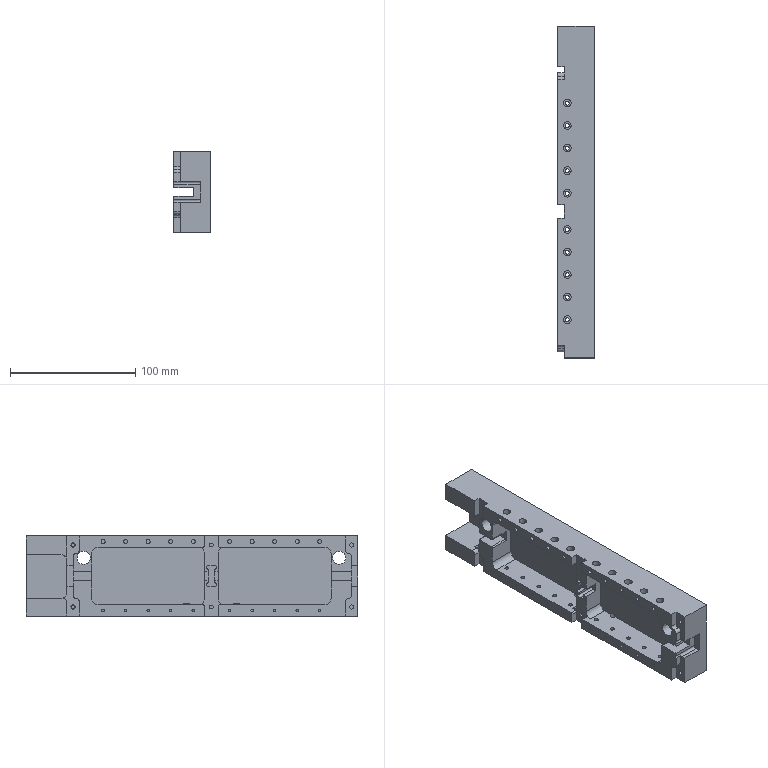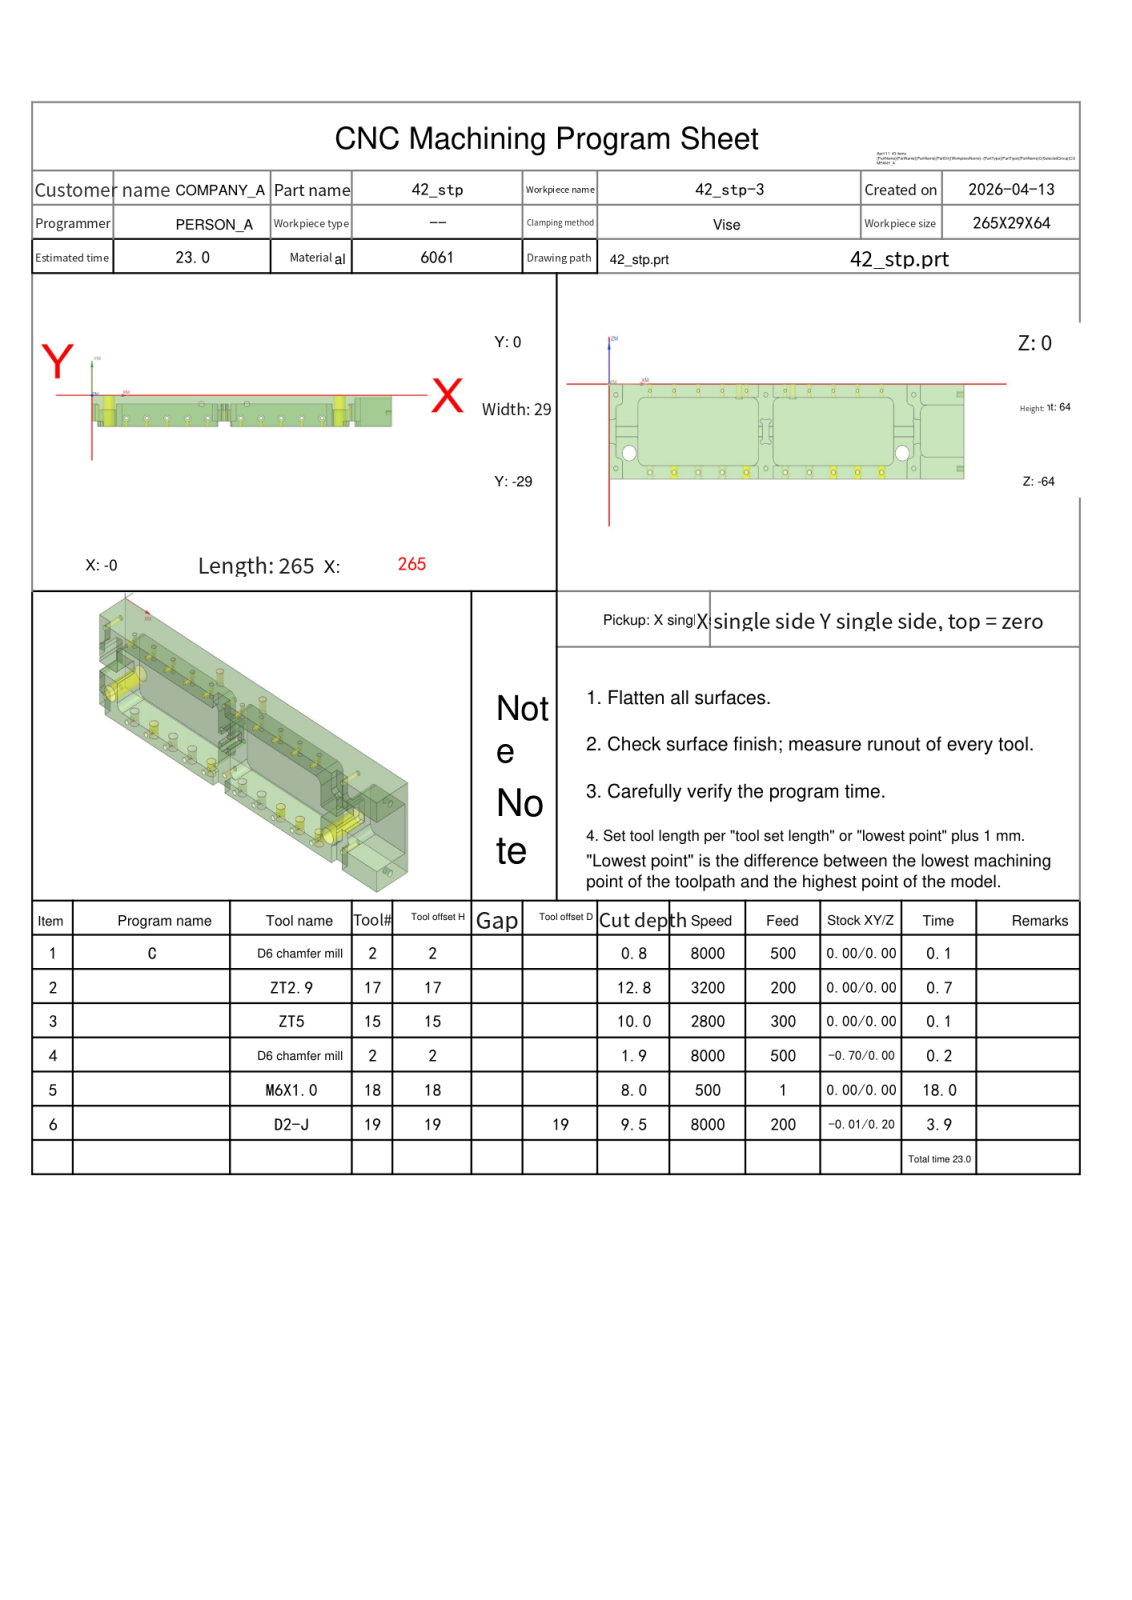NC program | NX | posted by the shop | part box 29 x 265 x 64 mm
Whole program:
%
O0001
(Machine time: 40.11 MIN)
(===Total Tool:5===)
(T2=D6 chamfer mill   D=6.   R=0.   D-  H02 Z=-1.85 )
(T17=ZT2.9  D=2.9  DR_a=120 D-  H17 Z=-12.84)
(T15=ZT5    D=5.   DR_a=118 D-  H15 Z=-10.  )
(T18=M6X1.0 D=5.   DR_a=180 D-  H18 Z=-8.   )
(T19=D2-J   D=2.   R=0.   D19 H19 Z=-9.5  )
G80 G90 G17 G49 G40
G91 G28 Z0
M01
N1 T02 M06
(D6 chamfer mill  D=6. R=0. H=02 ce=0.00 di=0.00)
G00 G90 G54 X203.5 Y-21.5 M03 S8000
G43 H02 Z20.
M08
G98 G81 X203.5 Y-21.5 Z-.8 R1. F500.
X185.5
X167.5
X149.5
X137. Y-8.003
X131.5 Y-21.5
X102.5
X97. Y-8.003
X84.5 Y-21.5
X66.5
X48.5
X30.5
G80
G00 Z20.
G91 G28 Z0.0
M05
M09
G91 G28 Z0.0
M01
N2 T17 M06
(ZT2.9 D=2.9 DR_a=120 H=17)
G00 G90 G54 X30.5 Y-21.5 M03 S3200
G43 H17 Z20.
M08
G98 G83 X30.5 Y-21.5 Z-12.837 R1. F200. Q2.
X48.5
X66.5
X84.5
X102.5
X131.5
X149.5
X167.5
X185.5
X203.5
G80
G00 Z20.
G91 G28 Z0.0
M05
M09
G91 G28 Z0.0
M01
N3 T15 M06
(ZT5 D=5. DR_a=118 H=15)
G00 G90 G54 X137. Y-8.003 M03 S2800
G43 H15 Z20.
M08
G98 G83 X137. Y-8.003 Z-10. R1. F300. Q2.
X97.
G80
G00 Z20.
G91 G28 Z0.0
M05
M09
G91 G28 Z0.0
M01
N4 T02 M06
(D6 chamfer mill  D=6. R=0. H=02 ce=0.00 di=0.00)
G00 G90 G54 X30.5 Y-21.5 M03 S8000
G43 H02 Z20.
M08
G98 G81 X30.5 Y-21.5 Z-1.85 R3. F500.
X48.5
X66.5
X84.5
X102.5
X131.5
X149.5
X167.5
X185.5
X203.5
G80
G00 Z20.
G00 G90 X136.051 Y-8.32 M03 S8000
Z20.
Z-.7
G01 Z-1.2 F500.
X135.5 Y-8.503
G03 X137. Y-10.003 I1.5 J0.0
X139. Y-8.003 I0.0 J2.
X137. Y-6.003 I-2. J0.0
X135. Y-8.003 I0.0 J-2.
X137. Y-10.003 I2. J0.0
X138.5 Y-8.503 I0.0 J1.5
G01 X137.949 Y-8.32
Z-.7
G00 Z20.
X96.051
Z-.7
G01 Z-1.2
X95.5 Y-8.503
G03 X97. Y-10.003 I1.5 J0.0
X99. Y-8.003 I0.0 J2.
X97. Y-6.003 I-2. J0.0
X95. Y-8.003 I0.0 J-2.
X97. Y-10.003 I2. J0.0
X98.5 Y-8.503 I0.0 J1.5
G01 X97.949 Y-8.32
Z-.7
G00 Z20.
G91 G28 Z0.0
M05
M09
G91 G28 Z0.0
M01
N5 T18 M06
(M6X1.0 D=5. DR_a=180 H=18)
G00 G90 G54 X137. Y-8.003 M03 S500
G43 H18 Z20.
M08
G95
G98 G84 X137. Y-8.003 Z-8. R1. F1. Q3.
X97.
G80
G94
G00 Z20.
G91 G28 Z0.0
M05
M09
G91 G28 Z0.0
M01
N6 T19 M06
(D2-J  D=2. R=0. H=19 ce=-0.01 di=0.20)
G00 G90 G54 X167.5 Y-21.5 M03 S8000
G43 H19 Z20.
M08
Z.5
G41 D19
G01 X167.655 Y-21.373 F200.
G03 X167.744 Y-21.184 I-.155 J.189
X167.5 Y-20.94 I-.244 J0.0
X167.5 Y-20.94 Z0.0 I0.0 J-.56
X167.5 Y-20.94 Z-.5 I0.0 J-.56
X167.5 Y-20.94 Z-1. I0.0 J-.56
X167.5 Y-20.94 Z-1.5 I0.0 J-.56
X167.5 Y-20.94 Z-2. I0.0 J-.56
X167.5 Y-20.94 Z-2.5 I0.0 J-.56
X167.5 Y-20.94 Z-3. I0.0 J-.56
X167.5 Y-20.94 Z-3.5 I0.0 J-.56
X167.5 Y-20.94 Z-4. I0.0 J-.56
X167.5 Y-20.94 Z-4.5 I0.0 J-.56
X167.5 Y-20.94 Z-5. I0.0 J-.56
X167.5 Y-20.94 Z-5.5 I0.0 J-.56
X167.5 Y-20.94 Z-6. I0.0 J-.56
X167.5 Y-20.94 Z-6.5 I0.0 J-.56
X167.5 Y-20.94 Z-7. I0.0 J-.56
X167.5 Y-20.94 Z-7.5 I0.0 J-.56
X167.5 Y-20.94 Z-8. I0.0 J-.56
X167.5 Y-20.94 Z-8.5 I0.0 J-.56
X167.5 Y-20.94 Z-9. I0.0 J-.56
X167.5 Y-20.94 Z-9.5 I0.0 J-.56
X166.94 Y-21.5 I0.0 J-.56
X167.5 Y-22.06 I.56 J0.0
X168.06 Y-21.5 I0.0 J.56
X167.5 Y-20.94 I-.56 J0.0
X167.256 Y-21.184 I0.0 J-.244
X167.345 Y-21.373 I.244 J0.0
G01 G40 X167.5 Y-21.5
G00 Z20.
X185.5
Z.5
G41 D19
G01 X185.655 Y-21.373
G03 X185.744 Y-21.184 I-.155 J.189
X185.5 Y-20.94 I-.244 J0.0
X185.5 Y-20.94 Z0.0 I0.0 J-.56
X185.5 Y-20.94 Z-.5 I0.0 J-.56
X185.5 Y-20.94 Z-1. I0.0 J-.56
X185.5 Y-20.94 Z-1.5 I0.0 J-.56
X185.5 Y-20.94 Z-2. I0.0 J-.56
X185.5 Y-20.94 Z-2.5 I0.0 J-.56
X185.5 Y-20.94 Z-3. I0.0 J-.56
X185.5 Y-20.94 Z-3.5 I0.0 J-.56
X185.5 Y-20.94 Z-4. I0.0 J-.56
X185.5 Y-20.94 Z-4.5 I0.0 J-.56
X185.5 Y-20.94 Z-5. I0.0 J-.56
X185.5 Y-20.94 Z-5.5 I0.0 J-.56
X185.5 Y-20.94 Z-6. I0.0 J-.56
X185.5 Y-20.94 Z-6.5 I0.0 J-.56
X185.5 Y-20.94 Z-7. I0.0 J-.56
X185.5 Y-20.94 Z-7.5 I0.0 J-.56
X185.5 Y-20.94 Z-8. I0.0 J-.56
X185.5 Y-20.94 Z-8.5 I0.0 J-.56
X185.5 Y-20.94 Z-9. I0.0 J-.56
X185.5 Y-20.94 Z-9.5 I0.0 J-.56
X184.94 Y-21.5 I0.0 J-.56
X185.5 Y-22.06 I.56 J0.0
X186.06 Y-21.5 I0.0 J.56
X185.5 Y-20.94 I-.56 J0.0
X185.256 Y-21.184 I0.0 J-.244
X185.345 Y-21.373 I.244 J0.0
G01 G40 X185.5 Y-21.5
G00 Z20.
X203.5
Z.5
G41 D19
G01 X203.655 Y-21.373
G03 X203.744 Y-21.184 I-.155 J.189
X203.5 Y-20.94 I-.244 J0.0
X203.5 Y-20.94 Z0.0 I0.0 J-.56
X203.5 Y-20.94 Z-.5 I0.0 J-.56
X203.5 Y-20.94 Z-1. I0.0 J-.56
X203.5 Y-20.94 Z-1.5 I0.0 J-.56
X203.5 Y-20.94 Z-2. I0.0 J-.56
X203.5 Y-20.94 Z-2.5 I0.0 J-.56
X203.5 Y-20.94 Z-3. I0.0 J-.56
X203.5 Y-20.94 Z-3.5 I0.0 J-.56
X203.5 Y-20.94 Z-4. I0.0 J-.56
X203.5 Y-20.94 Z-4.5 I0.0 J-.56
X203.5 Y-20.94 Z-5. I0.0 J-.56
X203.5 Y-20.94 Z-5.5 I0.0 J-.56
X203.5 Y-20.94 Z-6. I0.0 J-.56
X203.5 Y-20.94 Z-6.5 I0.0 J-.56
X203.5 Y-20.94 Z-7. I0.0 J-.56
X203.5 Y-20.94 Z-7.5 I0.0 J-.56
X203.5 Y-20.94 Z-8. I0.0 J-.56
X203.5 Y-20.94 Z-8.5 I0.0 J-.56
X203.5 Y-20.94 Z-9. I0.0 J-.56
X203.5 Y-20.94 Z-9.5 I0.0 J-.56
X202.94 Y-21.5 I0.0 J-.56
X203.5 Y-22.06 I.56 J0.0
X204.06 Y-21.5 I0.0 J.56
X203.5 Y-20.94 I-.56 J0.0
X203.256 Y-21.184 I0.0 J-.244
X203.345 Y-21.373 I.244 J0.0
G01 G40 X203.5 Y-21.5
G00 Z20.
X149.5
Z.5
G41 D19
G01 X149.655 Y-21.373
G03 X149.744 Y-21.184 I-.155 J.189
X149.5 Y-20.94 I-.244 J0.0
X149.5 Y-20.94 Z0.0 I0.0 J-.56
X149.5 Y-20.94 Z-.5 I0.0 J-.56
X149.5 Y-20.94 Z-1. I0.0 J-.56
X149.5 Y-20.94 Z-1.5 I0.0 J-.56
X149.5 Y-20.94 Z-2. I0.0 J-.56
X149.5 Y-20.94 Z-2.5 I0.0 J-.56
X149.5 Y-20.94 Z-3. I0.0 J-.56
X149.5 Y-20.94 Z-3.5 I0.0 J-.56
X149.5 Y-20.94 Z-4. I0.0 J-.56
X149.5 Y-20.94 Z-4.5 I0.0 J-.56
X149.5 Y-20.94 Z-5. I0.0 J-.56
X149.5 Y-20.94 Z-5.5 I0.0 J-.56
X149.5 Y-20.94 Z-6. I0.0 J-.56
X149.5 Y-20.94 Z-6.5 I0.0 J-.56
X149.5 Y-20.94 Z-7. I0.0 J-.56
X149.5 Y-20.94 Z-7.5 I0.0 J-.56
X149.5 Y-20.94 Z-8. I0.0 J-.56
X149.5 Y-20.94 Z-8.5 I0.0 J-.56
X149.5 Y-20.94 Z-9. I0.0 J-.56
X149.5 Y-20.94 Z-9.5 I0.0 J-.56
X148.94 Y-21.5 I0.0 J-.56
X149.5 Y-22.06 I.56 J0.0
X150.06 Y-21.5 I0.0 J.56
X149.5 Y-20.94 I-.56 J0.0
X149.256 Y-21.184 I0.0 J-.244
X149.345 Y-21.373 I.244 J0.0
G01 G40 X149.5 Y-21.5
G00 Z20.
X131.5
Z.5
G41 D19
G01 X131.655 Y-21.373
G03 X131.744 Y-21.184 I-.155 J.189
X131.5 Y-20.94 I-.244 J0.0
X131.5 Y-20.94 Z0.0 I0.0 J-.56
X131.5 Y-20.94 Z-.5 I0.0 J-.56
X131.5 Y-20.94 Z-1. I0.0 J-.56
X131.5 Y-20.94 Z-1.5 I0.0 J-.56
X131.5 Y-20.94 Z-2. I0.0 J-.56
X131.5 Y-20.94 Z-2.5 I0.0 J-.56
X131.5 Y-20.94 Z-3. I0.0 J-.56
X131.5 Y-20.94 Z-3.5 I0.0 J-.56
X131.5 Y-20.94 Z-4. I0.0 J-.56
X131.5 Y-20.94 Z-4.5 I0.0 J-.56
X131.5 Y-20.94 Z-5. I0.0 J-.56
X131.5 Y-20.94 Z-5.5 I0.0 J-.56
X131.5 Y-20.94 Z-6. I0.0 J-.56
X131.5 Y-20.94 Z-6.5 I0.0 J-.56
X131.5 Y-20.94 Z-7. I0.0 J-.56
X131.5 Y-20.94 Z-7.5 I0.0 J-.56
X131.5 Y-20.94 Z-8. I0.0 J-.56
X131.5 Y-20.94 Z-8.5 I0.0 J-.56
X131.5 Y-20.94 Z-9. I0.0 J-.56
X131.5 Y-20.94 Z-9.5 I0.0 J-.56
X130.94 Y-21.5 I0.0 J-.56
X131.5 Y-22.06 I.56 J0.0
X132.06 Y-21.5 I0.0 J.56
X131.5 Y-20.94 I-.56 J0.0
X131.256 Y-21.184 I0.0 J-.244
X131.345 Y-21.373 I.244 J0.0
G01 G40 X131.5 Y-21.5
G00 Z20.
X102.5
Z.5
G41 D19
G01 X102.655 Y-21.373
G03 X102.744 Y-21.184 I-.155 J.189
X102.5 Y-20.94 I-.244 J0.0
X102.5 Y-20.94 Z0.0 I0.0 J-.56
X102.5 Y-20.94 Z-.5 I0.0 J-.56
X102.5 Y-20.94 Z-1. I0.0 J-.56
X102.5 Y-20.94 Z-1.5 I0.0 J-.56
X102.5 Y-20.94 Z-2. I0.0 J-.56
X102.5 Y-20.94 Z-2.5 I0.0 J-.56
X102.5 Y-20.94 Z-3. I0.0 J-.56
X102.5 Y-20.94 Z-3.5 I0.0 J-.56
X102.5 Y-20.94 Z-4. I0.0 J-.56
X102.5 Y-20.94 Z-4.5 I0.0 J-.56
X102.5 Y-20.94 Z-5. I0.0 J-.56
X102.5 Y-20.94 Z-5.5 I0.0 J-.56
X102.5 Y-20.94 Z-6. I0.0 J-.56
X102.5 Y-20.94 Z-6.5 I0.0 J-.56
X102.5 Y-20.94 Z-7. I0.0 J-.56
X102.5 Y-20.94 Z-7.5 I0.0 J-.56
X102.5 Y-20.94 Z-8. I0.0 J-.56
X102.5 Y-20.94 Z-8.5 I0.0 J-.56
X102.5 Y-20.94 Z-9. I0.0 J-.56
X102.5 Y-20.94 Z-9.5 I0.0 J-.56
X101.94 Y-21.5 I0.0 J-.56
X102.5 Y-22.06 I.56 J0.0
X103.06 Y-21.5 I0.0 J.56
X102.5 Y-20.94 I-.56 J0.0
X102.256 Y-21.184 I0.0 J-.244
X102.345 Y-21.373 I.244 J0.0
G01 G40 X102.5 Y-21.5
G00 Z20.
X84.5
Z.5
G41 D19
G01 X84.655 Y-21.373
G03 X84.744 Y-21.184 I-.155 J.189
X84.5 Y-20.94 I-.244 J0.0
X84.5 Y-20.94 Z0.0 I0.0 J-.56
X84.5 Y-20.94 Z-.5 I0.0 J-.56
X84.5 Y-20.94 Z-1. I0.0 J-.56
X84.5 Y-20.94 Z-1.5 I0.0 J-.56
X84.5 Y-20.94 Z-2. I0.0 J-.56
X84.5 Y-20.94 Z-2.5 I0.0 J-.56
X84.5 Y-20.94 Z-3. I0.0 J-.56
X84.5 Y-20.94 Z-3.5 I0.0 J-.56
X84.5 Y-20.94 Z-4. I0.0 J-.56
X84.5 Y-20.94 Z-4.5 I0.0 J-.56
X84.5 Y-20.94 Z-5. I0.0 J-.56
X84.5 Y-20.94 Z-5.5 I0.0 J-.56
X84.5 Y-20.94 Z-6. I0.0 J-.56
X84.5 Y-20.94 Z-6.5 I0.0 J-.56
X84.5 Y-20.94 Z-7. I0.0 J-.56
X84.5 Y-20.94 Z-7.5 I0.0 J-.56
X84.5 Y-20.94 Z-8. I0.0 J-.56
X84.5 Y-20.94 Z-8.5 I0.0 J-.56
X84.5 Y-20.94 Z-9. I0.0 J-.56
X84.5 Y-20.94 Z-9.5 I0.0 J-.56
X83.94 Y-21.5 I0.0 J-.56
X84.5 Y-22.06 I.56 J0.0
X85.06 Y-21.5 I0.0 J.56
X84.5 Y-20.94 I-.56 J0.0
X84.256 Y-21.184 I0.0 J-.244
X84.345 Y-21.373 I.244 J0.0
G01 G40 X84.5 Y-21.5
G00 Z20.
X66.5
Z.5
G41 D19
G01 X66.655 Y-21.373
G03 X66.744 Y-21.184 I-.155 J.189
X66.5 Y-20.94 I-.244 J0.0
X66.5 Y-20.94 Z0.0 I0.0 J-.56
X66.5 Y-20.94 Z-.5 I0.0 J-.56
X66.5 Y-20.94 Z-1. I0.0 J-.56
X66.5 Y-20.94 Z-1.5 I0.0 J-.56
X66.5 Y-20.94 Z-2. I0.0 J-.56
X66.5 Y-20.94 Z-2.5 I0.0 J-.56
X66.5 Y-20.94 Z-3. I0.0 J-.56
X66.5 Y-20.94 Z-3.5 I0.0 J-.56
X66.5 Y-20.94 Z-4. I0.0 J-.56
X66.5 Y-20.94 Z-4.5 I0.0 J-.56
X66.5 Y-20.94 Z-5. I0.0 J-.56
X66.5 Y-20.94 Z-5.5 I0.0 J-.56
X66.5 Y-20.94 Z-6. I0.0 J-.56
X66.5 Y-20.94 Z-6.5 I0.0 J-.56
X66.5 Y-20.94 Z-7. I0.0 J-.56
X66.5 Y-20.94 Z-7.5 I0.0 J-.56
X66.5 Y-20.94 Z-8. I0.0 J-.56
X66.5 Y-20.94 Z-8.5 I0.0 J-.56
X66.5 Y-20.94 Z-9. I0.0 J-.56
X66.5 Y-20.94 Z-9.5 I0.0 J-.56
X65.94 Y-21.5 I0.0 J-.56
X66.5 Y-22.06 I.56 J0.0
X67.06 Y-21.5 I0.0 J.56
X66.5 Y-20.94 I-.56 J0.0
X66.256 Y-21.184 I0.0 J-.244
X66.345 Y-21.373 I.244 J0.0
G01 G40 X66.5 Y-21.5
G00 Z20.
X48.5
Z.5
G41 D19
G01 X48.655 Y-21.373
G03 X48.744 Y-21.184 I-.155 J.189
X48.5 Y-20.94 I-.244 J0.0
X48.5 Y-20.94 Z0.0 I0.0 J-.56
X48.5 Y-20.94 Z-.5 I0.0 J-.56
X48.5 Y-20.94 Z-1. I0.0 J-.56
X48.5 Y-20.94 Z-1.5 I0.0 J-.56
X48.5 Y-20.94 Z-2. I0.0 J-.56
X48.5 Y-20.94 Z-2.5 I0.0 J-.56
X48.5 Y-20.94 Z-3. I0.0 J-.56
X48.5 Y-20.94 Z-3.5 I0.0 J-.56
X48.5 Y-20.94 Z-4. I0.0 J-.56
X48.5 Y-20.94 Z-4.5 I0.0 J-.56
X48.5 Y-20.94 Z-5. I0.0 J-.56
X48.5 Y-20.94 Z-5.5 I0.0 J-.56
X48.5 Y-20.94 Z-6. I0.0 J-.56
X48.5 Y-20.94 Z-6.5 I0.0 J-.56
X48.5 Y-20.94 Z-7. I0.0 J-.56
X48.5 Y-20.94 Z-7.5 I0.0 J-.56
X48.5 Y-20.94 Z-8. I0.0 J-.56
X48.5 Y-20.94 Z-8.5 I0.0 J-.56
X48.5 Y-20.94 Z-9. I0.0 J-.56
X48.5 Y-20.94 Z-9.5 I0.0 J-.56
X47.94 Y-21.5 I0.0 J-.56
X48.5 Y-22.06 I.56 J0.0
X49.06 Y-21.5 I0.0 J.56
X48.5 Y-20.94 I-.56 J0.0
X48.256 Y-21.184 I0.0 J-.244
X48.345 Y-21.373 I.244 J0.0
G01 G40 X48.5 Y-21.5
G00 Z20.
X30.5
Z.5
G41 D19
G01 X30.655 Y-21.373
G03 X30.744 Y-21.184 I-.155 J.189
X30.5 Y-20.94 I-.244 J0.0
X30.5 Y-20.94 Z0.0 I0.0 J-.56
X30.5 Y-20.94 Z-.5 I0.0 J-.56
X30.5 Y-20.94 Z-1. I0.0 J-.56
X30.5 Y-20.94 Z-1.5 I0.0 J-.56
X30.5 Y-20.94 Z-2. I0.0 J-.56
X30.5 Y-20.94 Z-2.5 I0.0 J-.56
X30.5 Y-20.94 Z-3. I0.0 J-.56
X30.5 Y-20.94 Z-3.5 I0.0 J-.56
X30.5 Y-20.94 Z-4. I0.0 J-.56
X30.5 Y-20.94 Z-4.5 I0.0 J-.56
X30.5 Y-20.94 Z-5. I0.0 J-.56
X30.5 Y-20.94 Z-5.5 I0.0 J-.56
X30.5 Y-20.94 Z-6. I0.0 J-.56
X30.5 Y-20.94 Z-6.5 I0.0 J-.56
X30.5 Y-20.94 Z-7. I0.0 J-.56
X30.5 Y-20.94 Z-7.5 I0.0 J-.56
X30.5 Y-20.94 Z-8. I0.0 J-.56
X30.5 Y-20.94 Z-8.5 I0.0 J-.56
X30.5 Y-20.94 Z-9. I0.0 J-.56
X30.5 Y-20.94 Z-9.5 I0.0 J-.56
X29.94 Y-21.5 I0.0 J-.56
X30.5 Y-22.06 I.56 J0.0
X31.06 Y-21.5 I0.0 J.56
X30.5 Y-20.94 I-.56 J0.0
X30.256 Y-21.184 I0.0 J-.244
X30.345 Y-21.373 I.244 J0.0
G01 G40 X30.5 Y-21.5
G00 Z20.
M05
M09
G91 G28 Z0.0
G91 G28 Y0.0
M30
%